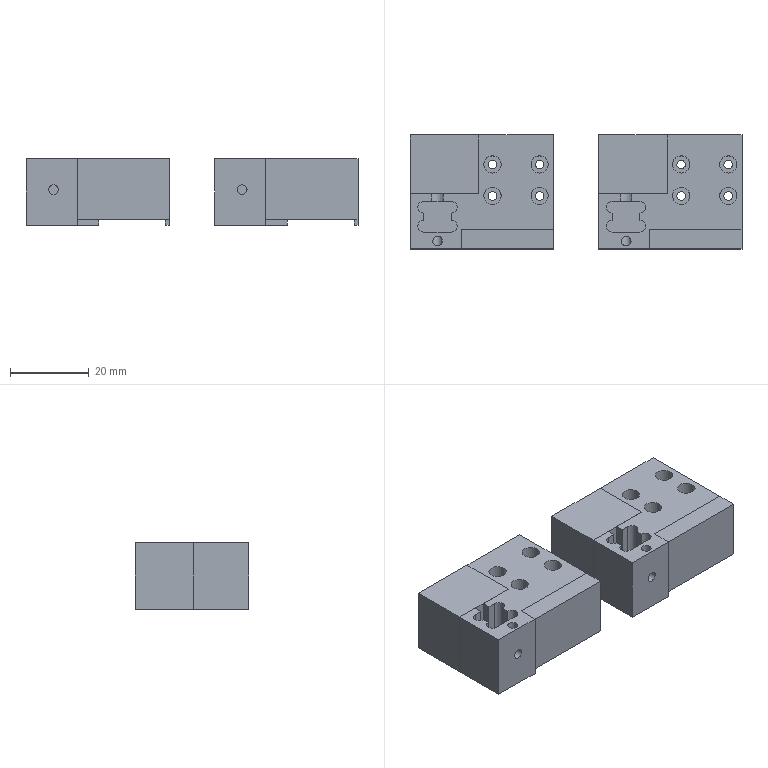Part | 6 solids | 128 faces | box 84.5 x 29 x 17 mm | volume 28338 mm3 | plane 74 | cylinder 42 | spline 12 | commonest cylinder face diameters 2.2 x8 2.5 x8 3 x8 4.399 x8 2.05 x6 4 x2